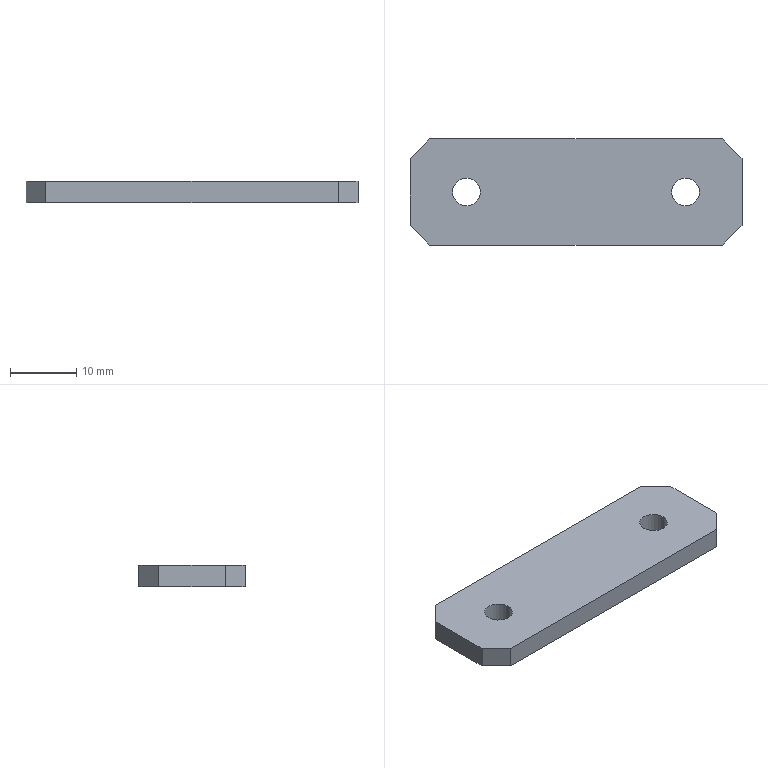Part | SolidWorks | features BaseBody 1 | 1 solid | 14 faces | box 50 x 16 x 3.2 mm | volume 2415 mm3 | plane 10 | cylinder 4 | commonest cylinder face diameters 4.17 x4
STEP:
#1=CARTESIAN_POINT('',(14.415,0.,3.2));
#2=VERTEX_POINT('',#1);
#3=CARTESIAN_POINT('',(18.585,0.,3.2));
#4=VERTEX_POINT('',#3);
#5=CARTESIAN_POINT('',(16.5,0.,3.2));
#6=DIRECTION('',(0.,0.,1.));
#7=DIRECTION('',(-1.,0.,0.));
#8=AXIS2_PLACEMENT_3D('',#5,#6,#7);
#9=CIRCLE('',#8,2.085);
#10=EDGE_CURVE('',#2,#4,#9,.T.);
#11=ORIENTED_EDGE('',*,*,#10,.T.);
#12=CARTESIAN_POINT('',(18.585,0.,0.));
#13=VERTEX_POINT('',#12);
#14=CARTESIAN_POINT('',(18.585,0.,3.2));
#15=DIRECTION('',(0.,0.,-1.));
#16=VECTOR('',#15,1000.);
#17=LINE('',#14,#16);
#18=EDGE_CURVE('',#4,#13,#17,.T.);
#19=ORIENTED_EDGE('',*,*,#18,.T.);
#20=CARTESIAN_POINT('',(14.415,0.,0.));
#21=VERTEX_POINT('',#20);
#22=CARTESIAN_POINT('',(16.5,0.,0.));
#23=DIRECTION('',(0.,0.,-1.));
#24=DIRECTION('',(-1.,0.,0.));
#25=AXIS2_PLACEMENT_3D('',#22,#23,#24);
#26=CIRCLE('',#25,2.085);
#27=EDGE_CURVE('',#13,#21,#26,.T.);
#28=ORIENTED_EDGE('',*,*,#27,.T.);
#29=CARTESIAN_POINT('',(14.415,0.,3.2));
#30=DIRECTION('',(0.,0.,-1.));
#31=VECTOR('',#30,1000.);
#32=LINE('',#29,#31);
#33=EDGE_CURVE('',#2,#21,#32,.T.);
#34=ORIENTED_EDGE('',*,*,#33,.F.);
#35=EDGE_LOOP('',(#11,#19,#28,#34));
#36=FACE_OUTER_BOUND('',#35,.T.);
#37=CARTESIAN_POINT('',(16.5,0.,3.2));
#38=DIRECTION('',(0.,0.,-1.));
#39=DIRECTION('',(-1.,0.,0.));
#40=AXIS2_PLACEMENT_3D('',#37,#38,#39);
#41=CYLINDRICAL_SURFACE('',#40,2.085);
#42=ADVANCED_FACE('',(#36),#41,.F.);
#43=CARTESIAN_POINT('',(-14.415,0.,3.2));
#44=VERTEX_POINT('',#43);
#45=CARTESIAN_POINT('',(-18.585,0.,3.2));
#46=VERTEX_POINT('',#45);
#47=CARTESIAN_POINT('',(-16.5,0.,3.2));
#48=DIRECTION('',(0.,0.,-1.));
#49=DIRECTION('',(-1.,0.,0.));
#50=AXIS2_PLACEMENT_3D('',#47,#48,#49);
#51=CIRCLE('',#50,2.085);
#52=EDGE_CURVE('',#44,#46,#51,.T.);
#53=ORIENTED_EDGE('',*,*,#52,.F.);
#54=CARTESIAN_POINT('',(-14.415,0.,0.));
#55=VERTEX_POINT('',#54);
#56=CARTESIAN_POINT('',(-14.415,0.,3.2));
#57=DIRECTION('',(0.,0.,-1.));
#58=VECTOR('',#57,1000.);
#59=LINE('',#56,#58);
#60=EDGE_CURVE('',#44,#55,#59,.T.);
#61=ORIENTED_EDGE('',*,*,#60,.T.);
#62=CARTESIAN_POINT('',(-18.585,0.,0.));
#63=VERTEX_POINT('',#62);
#64=CARTESIAN_POINT('',(-16.5,0.,0.));
#65=DIRECTION('',(0.,0.,-1.));
#66=DIRECTION('',(-1.,0.,0.));
#67=AXIS2_PLACEMENT_3D('',#64,#65,#66);
#68=CIRCLE('',#67,2.085);
#69=EDGE_CURVE('',#55,#63,#68,.T.);
#70=ORIENTED_EDGE('',*,*,#69,.T.);
#71=CARTESIAN_POINT('',(-18.585,0.,3.2));
#72=DIRECTION('',(0.,0.,-1.));
#73=VECTOR('',#72,1000.);
#74=LINE('',#71,#73);
#75=EDGE_CURVE('',#46,#63,#74,.T.);
#76=ORIENTED_EDGE('',*,*,#75,.F.);
#77=EDGE_LOOP('',(#53,#61,#70,#76));
#78=FACE_OUTER_BOUND('',#77,.T.);
#79=CARTESIAN_POINT('',(-16.5,0.,3.2));
#80=DIRECTION('',(0.,0.,-1.));
#81=DIRECTION('',(-1.,0.,0.));
#82=AXIS2_PLACEMENT_3D('',#79,#80,#81);
#83=CYLINDRICAL_SURFACE('',#82,2.085);
#84=ADVANCED_FACE('',(#78),#83,.F.);
#85=ORIENTED_EDGE('',*,*,#18,.F.);
#86=CARTESIAN_POINT('',(16.5,0.,3.2));
#87=DIRECTION('',(0.,0.,1.));
#88=DIRECTION('',(-1.,0.,0.));
#89=AXIS2_PLACEMENT_3D('',#86,#87,#88);
#90=CIRCLE('',#89,2.085);
#91=EDGE_CURVE('',#4,#2,#90,.T.);
#92=ORIENTED_EDGE('',*,*,#91,.T.);
#93=ORIENTED_EDGE('',*,*,#33,.T.);
#94=CARTESIAN_POINT('',(16.5,0.,0.));
#95=DIRECTION('',(0.,0.,-1.));
#96=DIRECTION('',(-1.,0.,0.));
#97=AXIS2_PLACEMENT_3D('',#94,#95,#96);
#98=CIRCLE('',#97,2.085);
#99=EDGE_CURVE('',#21,#13,#98,.T.);
#100=ORIENTED_EDGE('',*,*,#99,.T.);
#101=EDGE_LOOP('',(#85,#92,#93,#100));
#102=FACE_OUTER_BOUND('',#101,.T.);
#103=CARTESIAN_POINT('',(16.5,0.,3.2));
#104=DIRECTION('',(0.,0.,-1.));
#105=DIRECTION('',(-1.,0.,0.));
#106=AXIS2_PLACEMENT_3D('',#103,#104,#105);
#107=CYLINDRICAL_SURFACE('',#106,2.085);
#108=ADVANCED_FACE('',(#102),#107,.F.);
#109=CARTESIAN_POINT('',(-16.5,0.,0.));
#110=DIRECTION('',(0.,0.,-1.));
#111=DIRECTION('',(-1.,0.,0.));
#112=AXIS2_PLACEMENT_3D('',#109,#110,#111);
#113=CIRCLE('',#112,2.085);
#114=EDGE_CURVE('',#63,#55,#113,.T.);
#115=ORIENTED_EDGE('',*,*,#114,.F.);
#116=ORIENTED_EDGE('',*,*,#69,.F.);
#117=EDGE_LOOP('',(#115,#116));
#118=FACE_BOUND('',#117,.T.);
#119=ORIENTED_EDGE('',*,*,#99,.F.);
#120=ORIENTED_EDGE('',*,*,#27,.F.);
#121=EDGE_LOOP('',(#119,#120));
#122=FACE_BOUND('',#121,.T.);
#123=CARTESIAN_POINT('',(-25.,-5.,0.));
#124=VERTEX_POINT('',#123);
#125=CARTESIAN_POINT('',(-22.,-8.,0.));
#126=VERTEX_POINT('',#125);
#127=CARTESIAN_POINT('',(-22.,-8.,0.));
#128=DIRECTION('',(0.7071,-0.7071,0.));
#129=VECTOR('',#128,1000.);
#130=LINE('',#127,#129);
#131=EDGE_CURVE('',#124,#126,#130,.T.);
#132=ORIENTED_EDGE('',*,*,#131,.F.);
#133=CARTESIAN_POINT('',(-25.,5.,0.));
#134=VERTEX_POINT('',#133);
#135=CARTESIAN_POINT('',(-25.,0.,0.));
#136=DIRECTION('',(0.,-1.,0.));
#137=VECTOR('',#136,1000.);
#138=LINE('',#135,#137);
#139=EDGE_CURVE('',#134,#124,#138,.T.);
#140=ORIENTED_EDGE('',*,*,#139,.F.);
#141=CARTESIAN_POINT('',(-22.,8.,0.));
#142=VERTEX_POINT('',#141);
#143=CARTESIAN_POINT('',(-25.,5.,0.));
#144=DIRECTION('',(-0.7071,-0.7071,0.));
#145=VECTOR('',#144,1000.);
#146=LINE('',#143,#145);
#147=EDGE_CURVE('',#142,#134,#146,.T.);
#148=ORIENTED_EDGE('',*,*,#147,.F.);
#149=CARTESIAN_POINT('',(22.,8.,0.));
#150=VERTEX_POINT('',#149);
#151=CARTESIAN_POINT('',(0.,8.,0.));
#152=DIRECTION('',(-1.,0.,0.));
#153=VECTOR('',#152,1000.);
#154=LINE('',#151,#153);
#155=EDGE_CURVE('',#150,#142,#154,.T.);
#156=ORIENTED_EDGE('',*,*,#155,.F.);
#157=CARTESIAN_POINT('',(25.,5.,0.));
#158=VERTEX_POINT('',#157);
#159=CARTESIAN_POINT('',(22.,8.,0.));
#160=DIRECTION('',(-0.7071,0.7071,0.));
#161=VECTOR('',#160,1000.);
#162=LINE('',#159,#161);
#163=EDGE_CURVE('',#158,#150,#162,.T.);
#164=ORIENTED_EDGE('',*,*,#163,.F.);
#165=CARTESIAN_POINT('',(25.,-5.,0.));
#166=VERTEX_POINT('',#165);
#167=CARTESIAN_POINT('',(25.,0.,0.));
#168=DIRECTION('',(0.,1.,0.));
#169=VECTOR('',#168,1000.);
#170=LINE('',#167,#169);
#171=EDGE_CURVE('',#166,#158,#170,.T.);
#172=ORIENTED_EDGE('',*,*,#171,.F.);
#173=CARTESIAN_POINT('',(22.,-8.,0.));
#174=VERTEX_POINT('',#173);
#175=CARTESIAN_POINT('',(25.,-5.,0.));
#176=DIRECTION('',(0.7071,0.7071,0.));
#177=VECTOR('',#176,1000.);
#178=LINE('',#175,#177);
#179=EDGE_CURVE('',#174,#166,#178,.T.);
#180=ORIENTED_EDGE('',*,*,#179,.F.);
#181=CARTESIAN_POINT('',(0.,-8.,0.));
#182=DIRECTION('',(1.,0.,0.));
#183=VECTOR('',#182,1000.);
#184=LINE('',#181,#183);
#185=EDGE_CURVE('',#126,#174,#184,.T.);
#186=ORIENTED_EDGE('',*,*,#185,.F.);
#187=EDGE_LOOP('',(#132,#140,#148,#156,#164,#172,#180,#186));
#188=FACE_OUTER_BOUND('',#187,.T.);
#189=CARTESIAN_POINT('',(-25.,-8.,0.));
#190=DIRECTION('',(0.,0.,1.));
#191=DIRECTION('',(1.,0.,0.));
#192=AXIS2_PLACEMENT_3D('',#189,#190,#191);
#193=PLANE('',#192);
#194=ADVANCED_FACE('',(#118,#122,#188),#193,.F.);
#195=CARTESIAN_POINT('',(-16.5,0.,3.2));
#196=DIRECTION('',(0.,0.,-1.));
#197=DIRECTION('',(-1.,0.,0.));
#198=AXIS2_PLACEMENT_3D('',#195,#196,#197);
#199=CIRCLE('',#198,2.085);
#200=EDGE_CURVE('',#46,#44,#199,.T.);
#201=ORIENTED_EDGE('',*,*,#200,.T.);
#202=ORIENTED_EDGE('',*,*,#52,.T.);
#203=EDGE_LOOP('',(#201,#202));
#204=FACE_BOUND('',#203,.T.);
#205=ORIENTED_EDGE('',*,*,#10,.F.);
#206=ORIENTED_EDGE('',*,*,#91,.F.);
#207=EDGE_LOOP('',(#205,#206));
#208=FACE_BOUND('',#207,.T.);
#209=CARTESIAN_POINT('',(-25.,5.,3.2));
#210=VERTEX_POINT('',#209);
#211=CARTESIAN_POINT('',(-25.,-5.,3.2));
#212=VERTEX_POINT('',#211);
#213=CARTESIAN_POINT('',(-25.,0.,3.2));
#214=DIRECTION('',(0.,-1.,0.));
#215=VECTOR('',#214,1000.);
#216=LINE('',#213,#215);
#217=EDGE_CURVE('',#210,#212,#216,.T.);
#218=ORIENTED_EDGE('',*,*,#217,.T.);
#219=CARTESIAN_POINT('',(-22.,-8.,3.2));
#220=VERTEX_POINT('',#219);
#221=CARTESIAN_POINT('',(-25.,-5.,3.2));
#222=DIRECTION('',(0.7071,-0.7071,0.));
#223=VECTOR('',#222,1000.);
#224=LINE('',#221,#223);
#225=EDGE_CURVE('',#212,#220,#224,.T.);
#226=ORIENTED_EDGE('',*,*,#225,.T.);
#227=CARTESIAN_POINT('',(22.,-8.,3.2));
#228=VERTEX_POINT('',#227);
#229=CARTESIAN_POINT('',(0.,-8.,3.2));
#230=DIRECTION('',(1.,0.,0.));
#231=VECTOR('',#230,1000.);
#232=LINE('',#229,#231);
#233=EDGE_CURVE('',#220,#228,#232,.T.);
#234=ORIENTED_EDGE('',*,*,#233,.T.);
#235=CARTESIAN_POINT('',(25.,-5.,3.2));
#236=VERTEX_POINT('',#235);
#237=CARTESIAN_POINT('',(22.,-8.,3.2));
#238=DIRECTION('',(0.7071,0.7071,0.));
#239=VECTOR('',#238,1000.);
#240=LINE('',#237,#239);
#241=EDGE_CURVE('',#228,#236,#240,.T.);
#242=ORIENTED_EDGE('',*,*,#241,.T.);
#243=CARTESIAN_POINT('',(25.,5.,3.2));
#244=VERTEX_POINT('',#243);
#245=CARTESIAN_POINT('',(25.,0.,3.2));
#246=DIRECTION('',(0.,1.,0.));
#247=VECTOR('',#246,1000.);
#248=LINE('',#245,#247);
#249=EDGE_CURVE('',#236,#244,#248,.T.);
#250=ORIENTED_EDGE('',*,*,#249,.T.);
#251=CARTESIAN_POINT('',(22.,8.,3.2));
#252=VERTEX_POINT('',#251);
#253=CARTESIAN_POINT('',(25.,5.,3.2));
#254=DIRECTION('',(-0.7071,0.7071,0.));
#255=VECTOR('',#254,1000.);
#256=LINE('',#253,#255);
#257=EDGE_CURVE('',#244,#252,#256,.T.);
#258=ORIENTED_EDGE('',*,*,#257,.T.);
#259=CARTESIAN_POINT('',(-22.,8.,3.2));
#260=VERTEX_POINT('',#259);
#261=CARTESIAN_POINT('',(0.,8.,3.2));
#262=DIRECTION('',(-1.,0.,0.));
#263=VECTOR('',#262,1000.);
#264=LINE('',#261,#263);
#265=EDGE_CURVE('',#252,#260,#264,.T.);
#266=ORIENTED_EDGE('',*,*,#265,.T.);
#267=CARTESIAN_POINT('',(-22.,8.,3.2));
#268=DIRECTION('',(-0.7071,-0.7071,0.));
#269=VECTOR('',#268,1000.);
#270=LINE('',#267,#269);
#271=EDGE_CURVE('',#260,#210,#270,.T.);
#272=ORIENTED_EDGE('',*,*,#271,.T.);
#273=EDGE_LOOP('',(#218,#226,#234,#242,#250,#258,#266,#272));
#274=FACE_OUTER_BOUND('',#273,.T.);
#275=CARTESIAN_POINT('',(-25.,-8.,3.2));
#276=DIRECTION('',(0.,0.,1.));
#277=DIRECTION('',(1.,0.,0.));
#278=AXIS2_PLACEMENT_3D('',#275,#276,#277);
#279=PLANE('',#278);
#280=ADVANCED_FACE('',(#204,#208,#274),#279,.T.);
#281=ORIENTED_EDGE('',*,*,#60,.F.);
#282=ORIENTED_EDGE('',*,*,#200,.F.);
#283=ORIENTED_EDGE('',*,*,#75,.T.);
#284=ORIENTED_EDGE('',*,*,#114,.T.);
#285=EDGE_LOOP('',(#281,#282,#283,#284));
#286=FACE_OUTER_BOUND('',#285,.T.);
#287=CARTESIAN_POINT('',(-16.5,0.,3.2));
#288=DIRECTION('',(0.,0.,-1.));
#289=DIRECTION('',(-1.,0.,0.));
#290=AXIS2_PLACEMENT_3D('',#287,#288,#289);
#291=CYLINDRICAL_SURFACE('',#290,2.085);
#292=ADVANCED_FACE('',(#286),#291,.F.);
#293=CARTESIAN_POINT('',(22.,-8.,1.6));
#294=DIRECTION('',(0.,0.,-1.));
#295=VECTOR('',#294,1000.);
#296=LINE('',#293,#295);
#297=EDGE_CURVE('',#228,#174,#296,.T.);
#298=ORIENTED_EDGE('',*,*,#297,.F.);
#299=ORIENTED_EDGE('',*,*,#233,.F.);
#300=CARTESIAN_POINT('',(-22.,-8.,1.6));
#301=DIRECTION('',(0.,0.,1.));
#302=VECTOR('',#301,1000.);
#303=LINE('',#300,#302);
#304=EDGE_CURVE('',#126,#220,#303,.T.);
#305=ORIENTED_EDGE('',*,*,#304,.F.);
#306=ORIENTED_EDGE('',*,*,#185,.T.);
#307=EDGE_LOOP('',(#298,#299,#305,#306));
#308=FACE_OUTER_BOUND('',#307,.T.);
#309=CARTESIAN_POINT('',(22.,-8.,0.));
#310=DIRECTION('',(0.,1.,0.));
#311=DIRECTION('',(-1.,0.,0.));
#312=AXIS2_PLACEMENT_3D('',#309,#310,#311);
#313=PLANE('',#312);
#314=ADVANCED_FACE('',(#308),#313,.F.);
#315=ORIENTED_EDGE('',*,*,#304,.T.);
#316=ORIENTED_EDGE('',*,*,#225,.F.);
#317=CARTESIAN_POINT('',(-25.,-5.,1.6));
#318=DIRECTION('',(0.,0.,1.));
#319=VECTOR('',#318,1000.);
#320=LINE('',#317,#319);
#321=EDGE_CURVE('',#124,#212,#320,.T.);
#322=ORIENTED_EDGE('',*,*,#321,.F.);
#323=ORIENTED_EDGE('',*,*,#131,.T.);
#324=EDGE_LOOP('',(#315,#316,#322,#323));
#325=FACE_OUTER_BOUND('',#324,.T.);
#326=CARTESIAN_POINT('',(-22.,-8.,0.));
#327=DIRECTION('',(0.7071,0.7071,0.));
#328=DIRECTION('',(-0.7071,0.7071,0.));
#329=AXIS2_PLACEMENT_3D('',#326,#327,#328);
#330=PLANE('',#329);
#331=ADVANCED_FACE('',(#325),#330,.F.);
#332=ORIENTED_EDGE('',*,*,#321,.T.);
#333=ORIENTED_EDGE('',*,*,#217,.F.);
#334=CARTESIAN_POINT('',(-25.,5.,1.6));
#335=DIRECTION('',(0.,0.,1.));
#336=VECTOR('',#335,1000.);
#337=LINE('',#334,#336);
#338=EDGE_CURVE('',#134,#210,#337,.T.);
#339=ORIENTED_EDGE('',*,*,#338,.F.);
#340=ORIENTED_EDGE('',*,*,#139,.T.);
#341=EDGE_LOOP('',(#332,#333,#339,#340));
#342=FACE_OUTER_BOUND('',#341,.T.);
#343=CARTESIAN_POINT('',(-25.,-5.,0.));
#344=DIRECTION('',(1.,0.,0.));
#345=DIRECTION('',(0.,1.,0.));
#346=AXIS2_PLACEMENT_3D('',#343,#344,#345);
#347=PLANE('',#346);
#348=ADVANCED_FACE('',(#342),#347,.F.);
#349=ORIENTED_EDGE('',*,*,#338,.T.);
#350=ORIENTED_EDGE('',*,*,#271,.F.);
#351=CARTESIAN_POINT('',(-22.,8.,1.6));
#352=DIRECTION('',(0.,0.,1.));
#353=VECTOR('',#352,1000.);
#354=LINE('',#351,#353);
#355=EDGE_CURVE('',#142,#260,#354,.T.);
#356=ORIENTED_EDGE('',*,*,#355,.F.);
#357=ORIENTED_EDGE('',*,*,#147,.T.);
#358=EDGE_LOOP('',(#349,#350,#356,#357));
#359=FACE_OUTER_BOUND('',#358,.T.);
#360=CARTESIAN_POINT('',(-25.,5.,0.));
#361=DIRECTION('',(0.7071,-0.7071,0.));
#362=DIRECTION('',(0.7071,0.7071,0.));
#363=AXIS2_PLACEMENT_3D('',#360,#361,#362);
#364=PLANE('',#363);
#365=ADVANCED_FACE('',(#359),#364,.F.);
#366=ORIENTED_EDGE('',*,*,#355,.T.);
#367=ORIENTED_EDGE('',*,*,#265,.F.);
#368=CARTESIAN_POINT('',(22.,8.,1.6));
#369=DIRECTION('',(0.,0.,1.));
#370=VECTOR('',#369,1000.);
#371=LINE('',#368,#370);
#372=EDGE_CURVE('',#150,#252,#371,.T.);
#373=ORIENTED_EDGE('',*,*,#372,.F.);
#374=ORIENTED_EDGE('',*,*,#155,.T.);
#375=EDGE_LOOP('',(#366,#367,#373,#374));
#376=FACE_OUTER_BOUND('',#375,.T.);
#377=CARTESIAN_POINT('',(-22.,8.,0.));
#378=DIRECTION('',(0.,-1.,0.));
#379=DIRECTION('',(1.,0.,0.));
#380=AXIS2_PLACEMENT_3D('',#377,#378,#379);
#381=PLANE('',#380);
#382=ADVANCED_FACE('',(#376),#381,.F.);
#383=ORIENTED_EDGE('',*,*,#372,.T.);
#384=ORIENTED_EDGE('',*,*,#257,.F.);
#385=CARTESIAN_POINT('',(25.,5.,1.6));
#386=DIRECTION('',(0.,0.,1.));
#387=VECTOR('',#386,1000.);
#388=LINE('',#385,#387);
#389=EDGE_CURVE('',#158,#244,#388,.T.);
#390=ORIENTED_EDGE('',*,*,#389,.F.);
#391=ORIENTED_EDGE('',*,*,#163,.T.);
#392=EDGE_LOOP('',(#383,#384,#390,#391));
#393=FACE_OUTER_BOUND('',#392,.T.);
#394=CARTESIAN_POINT('',(22.,8.,0.));
#395=DIRECTION('',(-0.7071,-0.7071,0.));
#396=DIRECTION('',(0.7071,-0.7071,0.));
#397=AXIS2_PLACEMENT_3D('',#394,#395,#396);
#398=PLANE('',#397);
#399=ADVANCED_FACE('',(#393),#398,.F.);
#400=ORIENTED_EDGE('',*,*,#389,.T.);
#401=ORIENTED_EDGE('',*,*,#249,.F.);
#402=CARTESIAN_POINT('',(25.,-5.,1.6));
#403=DIRECTION('',(0.,0.,1.));
#404=VECTOR('',#403,1000.);
#405=LINE('',#402,#404);
#406=EDGE_CURVE('',#166,#236,#405,.T.);
#407=ORIENTED_EDGE('',*,*,#406,.F.);
#408=ORIENTED_EDGE('',*,*,#171,.T.);
#409=EDGE_LOOP('',(#400,#401,#407,#408));
#410=FACE_OUTER_BOUND('',#409,.T.);
#411=CARTESIAN_POINT('',(25.,5.,0.));
#412=DIRECTION('',(-1.,0.,0.));
#413=DIRECTION('',(0.,-1.,0.));
#414=AXIS2_PLACEMENT_3D('',#411,#412,#413);
#415=PLANE('',#414);
#416=ADVANCED_FACE('',(#410),#415,.F.);
#417=ORIENTED_EDGE('',*,*,#406,.T.);
#418=ORIENTED_EDGE('',*,*,#241,.F.);
#419=ORIENTED_EDGE('',*,*,#297,.T.);
#420=ORIENTED_EDGE('',*,*,#179,.T.);
#421=EDGE_LOOP('',(#417,#418,#419,#420));
#422=FACE_OUTER_BOUND('',#421,.T.);
#423=CARTESIAN_POINT('',(25.,-5.,0.));
#424=DIRECTION('',(-0.7071,0.7071,0.));
#425=DIRECTION('',(-0.7071,-0.7071,0.));
#426=AXIS2_PLACEMENT_3D('',#423,#424,#425);
#427=PLANE('',#426);
#428=ADVANCED_FACE('',(#422),#427,.F.);
#429=CLOSED_SHELL('',(#42,#84,#108,#194,#280,#292,#314,#331,#348,#365,#382,#399,#416,#428));
#430=MANIFOLD_SOLID_BREP('',#429);
#431=CARTESIAN_POINT('',(0.,0.,0.));
#432=DIRECTION('',(0.,0.,1.));
#433=DIRECTION('',(1.,0.,0.));
#434=AXIS2_PLACEMENT_3D('',#431,#432,#433);
#435=(LENGTH_UNIT()NAMED_UNIT(*)SI_UNIT(.MILLI.,.METRE.));
#436=UNCERTAINTY_MEASURE_WITH_UNIT(LENGTH_MEASURE(0.00001),#435,'','');
#437=(NAMED_UNIT(*)PLANE_ANGLE_UNIT()SI_UNIT($,.RADIAN.));
#438=(NAMED_UNIT(*)SI_UNIT($,.STERADIAN.)SOLID_ANGLE_UNIT());
#439=(GEOMETRIC_REPRESENTATION_CONTEXT(3)GLOBAL_UNCERTAINTY_ASSIGNED_CONTEXT((#436))GLOBAL_UNIT_ASSIGNED_CONTEXT((#435,#437,#438))REPRESENTATION_CONTEXT('',''));
#440=ADVANCED_BREP_SHAPE_REPRESENTATION('',(#430,#434),#439);